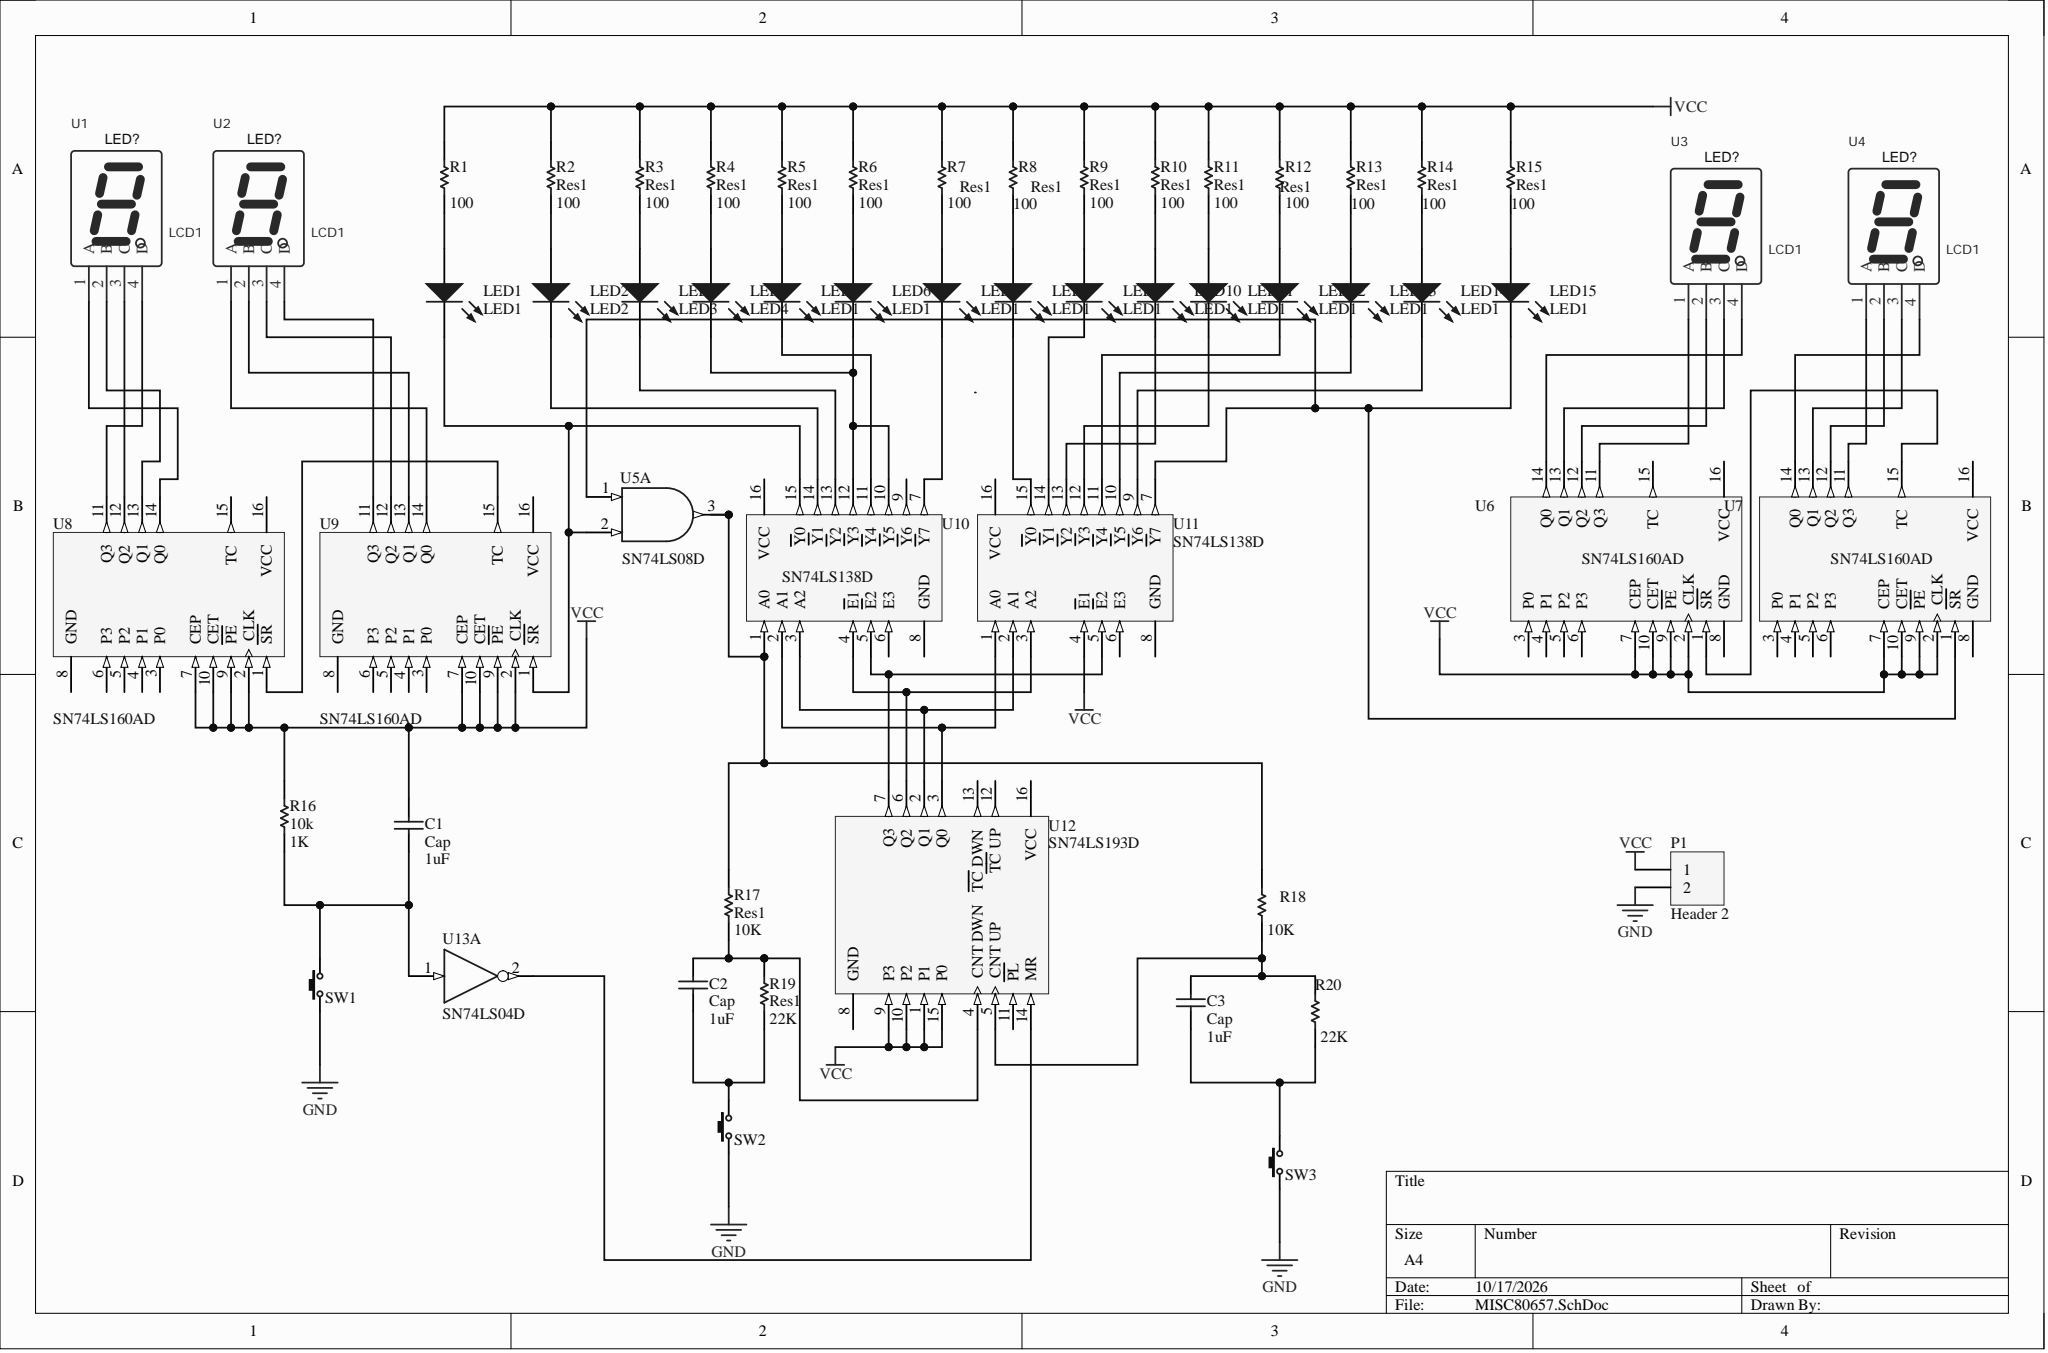Circuit board | Altium Designer | 55 parts | 60 nets
Bill of materials:
Comment,Description,Designator,Footprint,LibRef,Quantity
"Cap","Capacitor","C1, C2, C3","CS 2.0*5*8 - C","Cap","3"
"LED1","Typical BLUE SiC LED","LED1, LED5, LED6, LED7, LED8, LED9, LED10, LED11, LED12, LED13, LED14, LED15","LED 3MM-B","LED3","12"
"LED2","Typical BLUE SiC LED","LED2","LED 3MM-B","LED3","1"
"LED3","Typical BLUE SiC LED","LED3","LED 3MM-B","LED3","1"
"LED4","Typical BLUE SiC LED","LED4","LED 3MM-B","LED3","1"
"Header 2","Header, 2-Pin","P1","HDR1X2","Header 2","1"
"","Resistor","R1, R20","RS 1/4W","Res1","2"
"Res1","Resistor","R2, R3, R4, R5, R6, R7, R8, R9, R10, R11, R12, R13, R14, R15, R17, R18, R19","RS 1/4W","Res1","17"
"10k","Resistor","R16","RS 1/4W","Res1","1"
"3x6x5","3x6 tactile switch","SW1, SW2, SW3","TSW DIP-3*6*4.3","TSW 3x6","3"
"LCD1","","U1, U2, U3, U4","DCD-HEX","LCD1","4"
"SN74LS08D","Quad 2-Input AND Gate","U5","DIP14","SN74LS08D","1"
"SN74LS160AD","BCD Decade Counter","U6, U7, U8, U9","DIP16","SN74LS160AD","4"
"SN74LS138D","1-of-8 Decoder/Demultiplexer","U10, U11","DIP16","SN74LS138D","2"
"SN74LS193D","Presettable 4-Bit Binary Up/Down Counter","U12","DIP16","SN74LS193D","1"
"SN74LS04D","Hex Inverter","U13","DIP14","SN74LS04D","1"
Netlist (Protel format):
[
C1
CS 2.0*5*8 - C
Cap



]
[
C2
CS 2.0*5*8 - C
Cap



]
[
C3
CS 2.0*5*8 - C
Cap



]
[
LED1
LED 3MM-B
LED1



]
[
LED2
LED 3MM-B
LED2



]
[
LED3
LED 3MM-B
LED3



]
[
LED4
LED 3MM-B
LED4



]
[
LED5
LED 3MM-B
LED1



]
[
LED6
LED 3MM-B
LED1



]
[
LED7
LED 3MM-B
LED1



]
[
LED8
LED 3MM-B
LED1



]
[
LED9
LED 3MM-B
LED1



]
[
LED10
LED 3MM-B
LED1



]
[
LED11
LED 3MM-B
LED1



]
[
LED12
LED 3MM-B
LED1



]
[
LED13
LED 3MM-B
LED1



]
[
LED14
LED 3MM-B
LED1



]
[
LED15
LED 3MM-B
LED1



]
[
P1
HDR1X2
Header 2



]
[
R1
RS 1/4W




]
[
R2
RS 1/4W
Res1



]
[
R3
RS 1/4W
Res1



]
[
R4
RS 1/4W
Res1



]
[
R5
RS 1/4W
Res1



]
[
R6
RS 1/4W
Res1



]
[
R7
RS 1/4W
Res1



]
[
R8
RS 1/4W
Res1



]
[
R9
RS 1/4W
Res1



]
[
R10
RS 1/4W
Res1



]
[
R11
RS 1/4W
Res1



]
[
R12
RS 1/4W
Res1



]
[
R13
RS 1/4W
Res1



]
[
R14
RS 1/4W
Res1



]
[
R15
RS 1/4W
Res1



]
[
R16
RS 1/4W
10k



]
[
R17
RS 1/4W
Res1



]
[
R18
RS 1/4W
Res1



]
[
R19
RS 1/4W
Res1



]
[
R20
RS 1/4W




]
[
SW1
TSW DIP-3*6*4.3
3x6x5



]
[
SW2
TSW DIP-3*6*4.3
3x6x5



]
[
SW3
TSW DIP-3*6*4.3
3x6x5



]
[
U1
DCD-HEX
LCD1



]
[
U2
DCD-HEX
LCD1



]
[
U3
DCD-HEX
LCD1



]
[
U4
DCD-HEX
LCD1



]
[
U5
DIP14
SN74LS08D



]
[
U6
DIP16
SN74LS160AD



]
[
U7
DIP16
SN74LS160AD



]
[
U8
DIP16
SN74LS160AD



]
[
U9
DIP16
SN74LS160AD



]
[
U10
DIP16
SN74LS138D



]
[
U11
DIP16
SN74LS138D



]
[
U12
DIP16
SN74LS193D



]
[
U13
DIP14
SN74LS04D



]
(
VCC
C1-2
P1-1
R1-2
R2-2
R3-2
R4-2
R5-2
R6-2
R7-2
R8-2
R9-2
R10-2
R11-2
R12-2
R13-2
R14-2
R15-2
R16-2
U5-14
U6-2
U6-7
U6-9
U6-10
U7-2
U7-7
U7-9
U7-10
U8-2
U8-7
U8-9
U8-10
U9-2
U9-7
U9-9
U9-10
U11-4
U12-1
U12-9
U12-10
U12-15
)
(
NetU12_14
U12-14
U13-2
)
(
NetU10_5
U10-5
U11-5
U12-7
)
(
NetU10_4
U10-4
U11-3
U12-6
)
(
NetU10_3
U10-3
U11-2
U12-2
)
(
NetU10_2
U10-2
U11-1
U12-3
)
(
NetU8_1
U8-1
U9-15
)
(
NetU6_1
U6-1
U7-15
)
(
NetU4_4
U4-4
U7-14
)
(
NetU4_3
U4-3
U7-13
)
(
NetU4_2
U4-2
U7-12
)
(
NetU4_1
U4-1
U7-11
)
(
NetU3_4
U3-4
U6-14
)
(
NetU3_3
U3-3
U6-13
)
(
NetU3_2
U3-2
U6-12
)
(
NetU3_1
U3-1
U6-11
)
(
NetU2_4
U2-4
U9-11
)
(
NetU2_3
U2-3
U9-12
)
(
NetU2_2
U2-2
U9-13
)
(
NetU2_1
U2-1
U9-14
)
(
NetU1_4
U1-4
U8-11
)
(
NetU1_3
U1-3
U8-12
)
(
NetU1_2
U1-2
U8-13
)
(
NetU1_1
U1-1
U8-14
)
(
NetR17_2
R17-2
R18-2
U5-3
U10-1
)
(
NetLED15_2
LED15-2
U5-1
U7-1
U11-7
)
(
NetLED15_1
LED15-1
R15-1
)
(
NetLED14_2
LED14-2
U11-9
)
(
NetLED14_1
LED14-1
R14-1
)
(
NetLED13_2
LED13-2
U11-10
)
(
NetLED13_1
LED13-1
R13-1
)
(
NetLED12_2
LED12-2
U11-11
)
(
NetLED12_1
LED12-1
R12-1
)
(
NetLED11_2
LED11-2
U11-12
)
(
NetLED11_1
LED11-1
R11-1
)
(
NetLED10_2
LED10-2
U11-13
)
(
NetLED10_1
LED10-1
R10-1
)
(
NetLED9_2
LED9-2
U11-14
)
(
NetLED9_1
LED9-1
R9-1
)
(
NetLED8_2
LED8-2
U11-15
)
(
NetLED8_1
LED8-1
R8-1
)
(
NetLED7_2
LED7-2
U10-7
)
(
NetLED7_1
LED7-1
R7-1
)
(
NetLED6_1
LED6-1
R6-1
)
(
NetLED5_2
LED5-2
U10-11
)
(
NetLED5_1
LED5-1
R5-1
)
(
NetLED4_2
LED4-2
LED6-2
U10-10
U10-12
)
(
NetLED4_1
LED4-1
R4-1
)
(
NetLED3_2
LED3-2
U10-13
)
(
NetLED3_1
LED3-1
R3-1
)
(
NetLED2_2
LED2-2
U10-14
)
(
NetLED2_1
LED2-1
R2-1
)
(
NetLED1_2
LED1-2
U5-2
U9-1
U10-15
)
(
NetLED1_1
LED1-1
R1-1
)
(
NetC3_2
C3-2
R18-1
R20-2
U12-5
)
(
NetC3_1
C3-1
R20-1
SW3-2
)
(
NetC2_2
C2-2
R17-1
R19-2
U12-4
)
(
NetC2_1
C2-1
R19-1
SW2-2
)
(
NetC1_1
C1-1
R16-1
SW1-2
U13-1
)
(
GND
P1-2
SW1-1
SW2-1
SW3-1
U5-7
U13-7
)